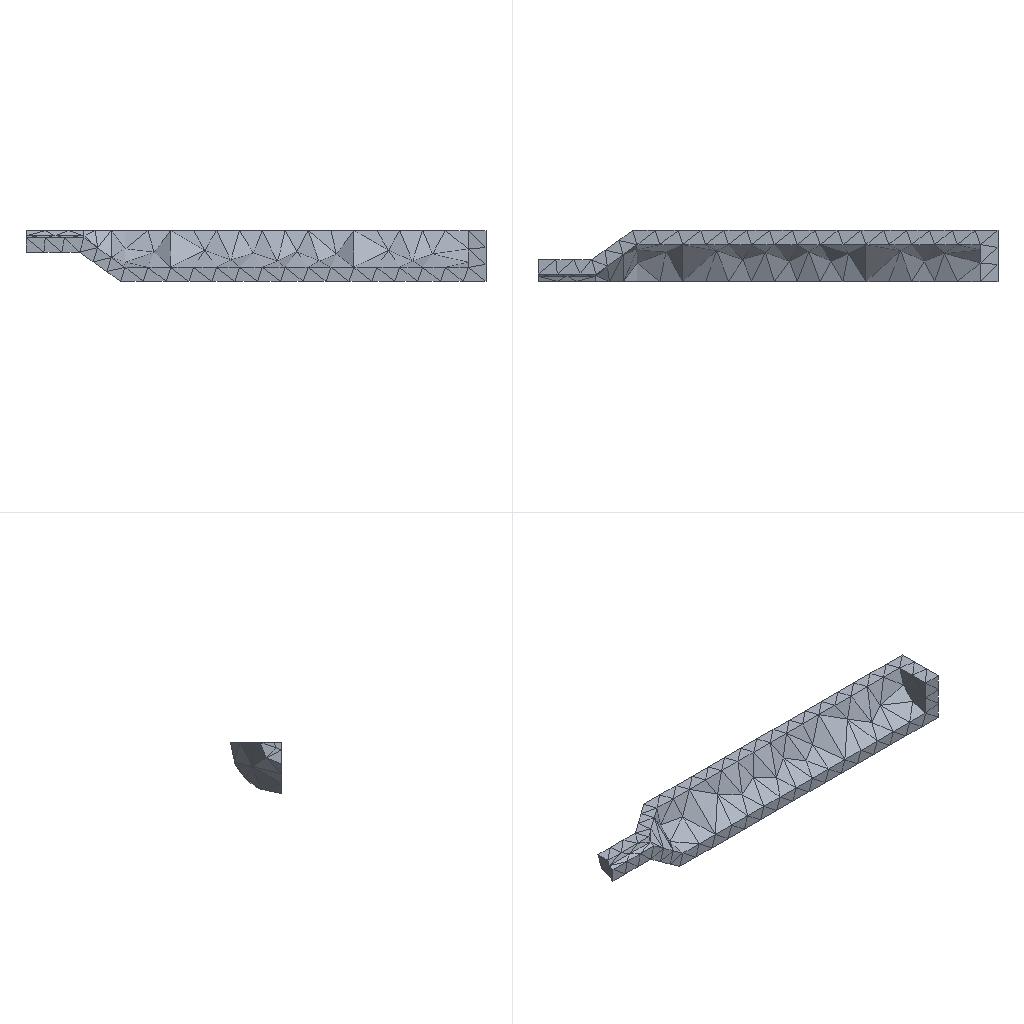Simulation study | ansys workbench
Ansys APDL input file, long lists of numbers shortened:
/batch
/config,noeldb,1     ! force off writing results to database
*get,_wallstrt,active,,time,wall
! ANSYS input file written by Workbench version 2022 R1
! File used for geometry attach:
/title,____--____ (C5)
! ****** Begin Custom Load Command Snippet ******
/COM, ACT Extensions:
/COM,     LSDYNA, 2021.1
/COM,
! ****** End   Custom Load Command Snippet ******
*DIM,_wb_ProjectScratch_dir,string,248
_wb_ProjectScratch_dir(1) = ''
*DIM,_wb_SolverFiles_dir,string,248
_wb_SolverFiles_dir(1) = ''
*DIM,_wb_userfiles_dir,string,248
_wb_userfiles_dir(1) = ''
/com,--- Data in consistent NMM units. See Solving Units in the help system for more information.
/units,MPA
/nopr
/wb,file,start              !  signify a WB generated input file
/prep7
! Turn off shape checking because checks already performed inside WB mesher.
! See help system for more information.
SHPP,OFF,,NOWARN
/nolist
etcon,set             ! allow ANSYS to choose best KEYOP's for 180x elements, resets any applicable keyopt to MAPDL defaults
/com,*********** Nodes for the whole assembly ***********
nblock,3,,834
(1i9,3e20.9e3)
        1     1.304000000E+03     1.443258926E+02     0.000000000E+00
! (758 more lines like these left out)
-1
/wb,elem,start            !  set before creation of elements
/com,*********** Elements for Body 1 "__3-FreeParts|__-__3" ***********
et,1,187
eblock,19,solid,,303
(19i9)
        1        1        1        1        0        0        0        0       10        0        1       41      138       42      104      361      366      357      359
! (605 more lines like these left out)
-1
/wb,elem,end               !  done creating elements
/com,*********** Send User Defined Coordinate System(s) ***********
csys,0
toffst,273.15,  ! Temperature offset from absolute zero
/com,*********** Set Reference Temperature ***********
tref,22.
/wb,mat,start              !  starting to send materials
/com,*********** Send Materials ***********
Temperature = 'TEMP' ! Temperature
MP,DENS,1,7.85e-09,	! tonne mm^-3
MP,ALPX,1,1.2e-05,	! C^-1
MP,C,1,434000000,	! mm^2 s^-2 C^-1
MP,KXX,1,60.5,	! tonne mm s^-3 C^-1
MP,RSVX,1,0.00017,	! ohm mm
MP,EX,1,200000,	! tonne s^-2 mm^-1
MP,NUXY,1,0.3,
MP,MURX,1,10000,
/wb,mat,end                !  done sending materials
!************************* Model Summary ********************
!__3-FreeParts|__-__3,	结构钢,	matid,	1
!************************* End Model Summary ********************
! get the diagonal of the bounding box. Needed later for other things
*get,_xmin,node,,mnloc,x
*get,_ymin,node,,mnloc,y
*get,_zmin,node,,mnloc,z
*get,_xmax,node,,mxloc,x
*get,_ymax,node,,mxloc,y
*get,_zmax,node,,mxloc,z
_ASMDIAG=(_xmax-_xmin)*(_xmax-_xmin)+(_ymax-_ymin)*(_ymax-_ymin)+(_zmax-_zmin)*(_zmax-_zmin)
_ASMDIAG=SQRT(_ASMDIAG)
/wb,contact,start          !  starting to send contact
/wb,contact,end            !  done creating contacts
/golist
/wb,load,start             !  starting to send loads
/com,*********** Fixed Supports ***********
CMBLOCK,_FIXEDSU,NODE,      147
(8i10)
         1         6         7         8        11        16        17        18
! (18 more lines like these left out)
cmsel,s,_FIXEDSU
d,all,all
nsel,all
/com,*********** Define Pressure Using Surface Effect Elements "__" ***********
et,2,154
eblock,10,,,56
(15i9)
      606        2        2        2        0       70       76       79       79      479      497       79      480
! (55 more lines like these left out)
-1
esel,s,type,,2
keyop,2,7,0                ! Use deformed area for application of load
esel,all
/com,*********** Define Pressure Using Surface Effect Elements "__ 2" ***********
et,3,154
eblock,10,,,94
(15i9)
      662        3        3        3        0        3      147       30       30      167      303       30      164
! (93 more lines like these left out)
-1
esel,s,type,,3
keyop,3,7,0                ! Use deformed area for application of load
esel,all
esel,all
/gst,on,on
fini
*get,_numnode,node,0,count
*get,_numelem,elem,0,count
*get, _MAXELEMNUM, elem, 0, NUM, MAX
*get, _MAXNODENUM, node, 0, NUM, MAX
*get, _MAXELEMTYPE, etyp, 0, NUM, MAX
*get, _MAXREALCONST, real, 0, NUM, MAX
/go
/wb,load,end               !  done creating loads
/com,--- Number of total nodes = %_numnode%
/com,--- Number of contact elements = 150
/com,--- Number of spring elements = 0
/com,--- Number of bearing elements = 0
/com,--- Number of solid elements = 303
/com,--- Number of condensed parts = 0
/com,--- Number of total elements = %_numelem%
*get,_wallbsol,active,,time,wall
/com,****************************************************************************
/com,*************************    SOLUTION       ********************************
/com,****************************************************************************
/solu
antype,0                   ! static analysis
_thickRatio=  0     ! Ratio of thick parts in the model
eqsl,sparse,,,,,1
cntr,print,1               ! print out contact info and also make no initial contact an error
dmpoption,emat,no             ! Don't combine emat file for DANSYS
dmpoption,esav,no             ! Don't combine esav file for DANSYS
nldiag,cont,iter           ! print out contact info each equilibrium iteration
rescontrol,,none                 ! Do not keep any restart files
/com,****************************************************
/com,******************* SOLVE FOR LS 1 OF 1 ****************
esel,s,type,,2
nsle
sf,all,pres,30.
esel,s,type,,3
nsle
sf,all,pres,20.
nsel,all
esel,all
esel,all
/nopr
/gopr
nsub,1,1,1
time,1.
outres,erase
outres,all,none
outres,nsol,all,
outres,rsol,all
outres,eangl,all
outres,etmp,all
outres,veng,all
outres,strs,all,
outres,epel,all,
outres,eppl,all,
outres,cont,all,
! *********** WB SOLVE COMMAND ***********
! check interactive state
*get,ANSINTER_,active,,int
*if,ANSINTER_,ne,0,then
/eof
*endif
solve
/com *************** Write FE CONNECTORS *********
CEWRITE,file,ce,,INTE
/com,****************************************************
/com,*************** FINISHED SOLVE FOR LS 1 *************
*get,_wallasol,active,,time,wall
/nopr
*get,_numnode,node,0,count
*get,_numelem,elem,0,count
*get, _MAXELEMNUM, elem, 0, NUM, MAX
*get, _MAXNODENUM, node, 0, NUM, MAX,,,INTERNAL
*get, _MAXELEMTYPE, etyp, 0, NUM, MAX
*get, _MAXREALCONST, real, 0, NUM, MAX
/gopr
/post1
xmlo,ENCODING,ISO-8859-1
xmlo,parm
/xml,parm,xml
fini
/gopr
*get,_walldone,active,,time,wall
_preptime=(_wallbsol-_wallstrt)*3600
_solvtime=(_wallasol-_wallbsol)*3600
_posttime=(_walldone-_wallasol)*3600
_totaltim=(_walldone-_wallstrt)*3600
*get,_dlbratio,active,0,solu,dlbr
*get,_combtime,active,0,solu,comb
*get,_ssmode,active,0,solu,ssmm
*get,_ndofs,active,0,solu,ndof
*get,_sol_end_time,active,0,set,time
*if,_sol_end_time,eq,1.,then
/fclean				!clean distributed files
*endif
/com,--- Total number of nodes = %_numnode%
/com,--- Total number of elements = %_numelem%
/com,--- Element load balance ratio = %_dlbratio%
/com,--- Time to combine distributed files = %_combtime%
/com,--- Sparse memory mode = %_ssmode%
/com,--- Number of DOF = %_ndofs%
/wb,file,end               ! done with WB generated input